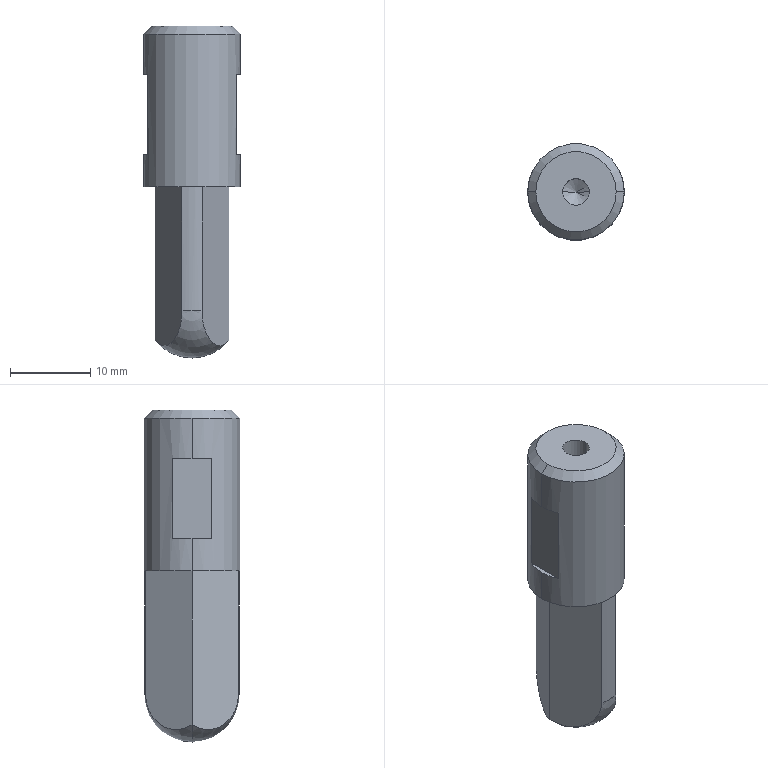Part | SolidWorks | features ICE 3, Chamfer 1, Extrusion 1, HoleWzd 1, Revolution 1 | 1 solid | 24 faces | box 12 x 12 x 41.3 mm | volume 3482 mm3 | plane 12 | cylinder 6 | cone 4 | sphere 2 | commonest cylinder face diameters 3.3 x2 11.8 x2 12 x2
STEP:
#1=CARTESIAN_POINT('',(5.,0.,35.4));
#2=VERTEX_POINT('',#1);
#3=CARTESIAN_POINT('',(-5.,0.,35.4));
#4=VERTEX_POINT('',#3);
#5=CARTESIAN_POINT('',(0.,0.,35.4));
#6=DIRECTION('',(0.,0.,1.));
#7=DIRECTION('',(1.,0.,0.));
#8=AXIS2_PLACEMENT_3D('',#5,#6,#7);
#9=CIRCLE('',#8,5.);
#10=EDGE_CURVE('',#2,#4,#9,.T.);
#11=ORIENTED_EDGE('',*,*,#10,.F.);
#12=CARTESIAN_POINT('',(6.,0.,34.4));
#13=VERTEX_POINT('',#12);
#14=CARTESIAN_POINT('',(5.,0.,35.4));
#15=DIRECTION('',(0.7071,0.,-0.7071));
#16=VECTOR('',#15,1000.);
#17=LINE('',#14,#16);
#18=EDGE_CURVE('',#2,#13,#17,.T.);
#19=ORIENTED_EDGE('',*,*,#18,.T.);
#20=CARTESIAN_POINT('',(-6.,0.,34.4));
#21=VERTEX_POINT('',#20);
#22=CARTESIAN_POINT('',(0.,0.,34.4));
#23=DIRECTION('',(0.,0.,-1.));
#24=DIRECTION('',(1.,0.,0.));
#25=AXIS2_PLACEMENT_3D('',#22,#23,#24);
#26=CIRCLE('',#25,6.);
#27=EDGE_CURVE('',#21,#13,#26,.T.);
#28=ORIENTED_EDGE('',*,*,#27,.F.);
#29=CARTESIAN_POINT('',(-5.,0.,35.4));
#30=DIRECTION('',(-0.7071,0.,-0.7071));
#31=VECTOR('',#30,1000.);
#32=LINE('',#29,#31);
#33=EDGE_CURVE('',#4,#21,#32,.T.);
#34=ORIENTED_EDGE('',*,*,#33,.F.);
#35=EDGE_LOOP('',(#11,#19,#28,#34));
#36=FACE_OUTER_BOUND('',#35,.T.);
#37=CARTESIAN_POINT('',(0.,0.,35.4));
#38=DIRECTION('',(0.,0.,-1.));
#39=DIRECTION('',(-1.,0.,0.));
#40=AXIS2_PLACEMENT_3D('',#37,#38,#39);
#41=CONICAL_SURFACE('',#40,5.,0.7854);
#42=ADVANCED_FACE('',(#36),#41,.T.);
#43=CARTESIAN_POINT('',(4.579,0.,-3.721));
#44=VERTEX_POINT('',#43);
#45=CARTESIAN_POINT('',(1.25,5.766,0.));
#46=VERTEX_POINT('',#45);
#47=CARTESIAN_POINT('',(3.434,1.983,0.));
#48=DIRECTION('',(0.866,0.5,0.));
#49=DIRECTION('',(0.5,-0.866,0.));
#50=AXIS2_PLACEMENT_3D('',#47,#48,#49);
#51=CIRCLE('',#50,4.369);
#52=EDGE_CURVE('',#44,#46,#51,.T.);
#53=ORIENTED_EDGE('',*,*,#52,.F.);
#54=CARTESIAN_POINT('',(0.,0.,-5.9));
#55=VERTEX_POINT('',#54);
#56=CARTESIAN_POINT('',(0.,0.,0.));
#57=DIRECTION('',(0.,1.,0.));
#58=DIRECTION('',(-1.,0.,0.));
#59=AXIS2_PLACEMENT_3D('',#56,#57,#58);
#60=CIRCLE('',#59,5.9);
#61=EDGE_CURVE('',#44,#55,#60,.T.);
#62=ORIENTED_EDGE('',*,*,#61,.T.);
#63=CARTESIAN_POINT('',(-4.579,0.,-3.721));
#64=VERTEX_POINT('',#63);
#65=CARTESIAN_POINT('',(0.,0.,0.));
#66=DIRECTION('',(0.,-1.,0.));
#67=DIRECTION('',(0.,0.,-1.));
#68=AXIS2_PLACEMENT_3D('',#65,#66,#67);
#69=CIRCLE('',#68,5.9);
#70=EDGE_CURVE('',#64,#55,#69,.T.);
#71=ORIENTED_EDGE('',*,*,#70,.F.);
#72=CARTESIAN_POINT('',(-1.25,5.766,0.));
#73=VERTEX_POINT('',#72);
#74=CARTESIAN_POINT('',(-3.434,1.983,0.));
#75=DIRECTION('',(-0.866,0.5,0.));
#76=DIRECTION('',(0.5,0.866,0.));
#77=AXIS2_PLACEMENT_3D('',#74,#75,#76);
#78=CIRCLE('',#77,4.369);
#79=EDGE_CURVE('',#73,#64,#78,.T.);
#80=ORIENTED_EDGE('',*,*,#79,.F.);
#81=CARTESIAN_POINT('',(0.,0.,0.));
#82=DIRECTION('',(0.,0.,-1.));
#83=DIRECTION('',(-1.,0.,0.));
#84=AXIS2_PLACEMENT_3D('',#81,#82,#83);
#85=CIRCLE('',#84,5.9);
#86=EDGE_CURVE('',#73,#46,#85,.T.);
#87=ORIENTED_EDGE('',*,*,#86,.T.);
#88=EDGE_LOOP('',(#53,#62,#71,#80,#87));
#89=FACE_OUTER_BOUND('',#88,.T.);
#90=CARTESIAN_POINT('',(0.,0.,0.));
#91=DIRECTION('',(0.,1.,0.));
#92=DIRECTION('',(-1.,0.,0.));
#93=AXIS2_PLACEMENT_3D('',#90,#91,#92);
#94=SPHERICAL_SURFACE('',#93,5.9);
#95=ADVANCED_FACE('',(#89),#94,.T.);
#96=CARTESIAN_POINT('',(6.,0.,15.4));
#97=VERTEX_POINT('',#96);
#98=CARTESIAN_POINT('',(-6.,0.,15.4));
#99=VERTEX_POINT('',#98);
#100=CARTESIAN_POINT('',(0.,0.,15.4));
#101=DIRECTION('',(0.,0.,1.));
#102=DIRECTION('',(1.,0.,0.));
#103=AXIS2_PLACEMENT_3D('',#100,#101,#102);
#104=CIRCLE('',#103,6.);
#105=EDGE_CURVE('',#97,#99,#104,.T.);
#106=ORIENTED_EDGE('',*,*,#105,.T.);
#107=CARTESIAN_POINT('',(-6.,0.,19.4));
#108=VERTEX_POINT('',#107);
#109=CARTESIAN_POINT('',(-6.,0.,15.4));
#110=DIRECTION('',(0.,0.,1.));
#111=VECTOR('',#110,1000.);
#112=LINE('',#109,#111);
#113=EDGE_CURVE('',#99,#108,#112,.T.);
#114=ORIENTED_EDGE('',*,*,#113,.T.);
#115=CARTESIAN_POINT('',(-5.5,2.398,19.4));
#116=VERTEX_POINT('',#115);
#117=CARTESIAN_POINT('',(0.,0.,19.4));
#118=DIRECTION('',(0.,0.,1.));
#119=DIRECTION('',(-1.,0.,0.));
#120=AXIS2_PLACEMENT_3D('',#117,#118,#119);
#121=CIRCLE('',#120,6.);
#122=EDGE_CURVE('',#116,#108,#121,.T.);
#123=ORIENTED_EDGE('',*,*,#122,.F.);
#124=CARTESIAN_POINT('',(-5.5,2.398,29.4));
#125=VERTEX_POINT('',#124);
#126=CARTESIAN_POINT('',(-5.5,2.398,15.4));
#127=DIRECTION('',(0.,0.,-1.));
#128=VECTOR('',#127,1000.);
#129=LINE('',#126,#128);
#130=EDGE_CURVE('',#125,#116,#129,.T.);
#131=ORIENTED_EDGE('',*,*,#130,.F.);
#132=CARTESIAN_POINT('',(-6.,0.,29.4));
#133=VERTEX_POINT('',#132);
#134=CARTESIAN_POINT('',(0.,0.,29.4));
#135=DIRECTION('',(0.,0.,-1.));
#136=DIRECTION('',(1.,0.,0.));
#137=AXIS2_PLACEMENT_3D('',#134,#135,#136);
#138=CIRCLE('',#137,6.);
#139=EDGE_CURVE('',#133,#125,#138,.T.);
#140=ORIENTED_EDGE('',*,*,#139,.F.);
#141=CARTESIAN_POINT('',(-6.,0.,15.4));
#142=DIRECTION('',(0.,0.,1.));
#143=VECTOR('',#142,1000.);
#144=LINE('',#141,#143);
#145=EDGE_CURVE('',#133,#21,#144,.T.);
#146=ORIENTED_EDGE('',*,*,#145,.T.);
#147=ORIENTED_EDGE('',*,*,#27,.T.);
#148=CARTESIAN_POINT('',(6.,0.,29.4));
#149=VERTEX_POINT('',#148);
#150=CARTESIAN_POINT('',(6.,0.,15.4));
#151=DIRECTION('',(0.,0.,1.));
#152=VECTOR('',#151,1000.);
#153=LINE('',#150,#152);
#154=EDGE_CURVE('',#149,#13,#153,.T.);
#155=ORIENTED_EDGE('',*,*,#154,.F.);
#156=CARTESIAN_POINT('',(5.5,2.398,29.4));
#157=VERTEX_POINT('',#156);
#158=CARTESIAN_POINT('',(0.,0.,29.4));
#159=DIRECTION('',(0.,0.,-1.));
#160=DIRECTION('',(1.,0.,0.));
#161=AXIS2_PLACEMENT_3D('',#158,#159,#160);
#162=CIRCLE('',#161,6.);
#163=EDGE_CURVE('',#157,#149,#162,.T.);
#164=ORIENTED_EDGE('',*,*,#163,.F.);
#165=CARTESIAN_POINT('',(5.5,2.398,19.4));
#166=VERTEX_POINT('',#165);
#167=CARTESIAN_POINT('',(5.5,2.398,15.4));
#168=DIRECTION('',(0.,0.,1.));
#169=VECTOR('',#168,1000.);
#170=LINE('',#167,#169);
#171=EDGE_CURVE('',#166,#157,#170,.T.);
#172=ORIENTED_EDGE('',*,*,#171,.F.);
#173=CARTESIAN_POINT('',(6.,0.,19.4));
#174=VERTEX_POINT('',#173);
#175=CARTESIAN_POINT('',(0.,0.,19.4));
#176=DIRECTION('',(0.,0.,1.));
#177=DIRECTION('',(-1.,0.,0.));
#178=AXIS2_PLACEMENT_3D('',#175,#176,#177);
#179=CIRCLE('',#178,6.);
#180=EDGE_CURVE('',#174,#166,#179,.T.);
#181=ORIENTED_EDGE('',*,*,#180,.F.);
#182=CARTESIAN_POINT('',(6.,0.,15.4));
#183=DIRECTION('',(0.,0.,1.));
#184=VECTOR('',#183,1000.);
#185=LINE('',#182,#184);
#186=EDGE_CURVE('',#97,#174,#185,.T.);
#187=ORIENTED_EDGE('',*,*,#186,.F.);
#188=EDGE_LOOP('',(#106,#114,#123,#131,#140,#146,#147,#155,#164,#172,#181,#187));
#189=FACE_OUTER_BOUND('',#188,.T.);
#190=CARTESIAN_POINT('',(0.,0.,15.4));
#191=DIRECTION('',(0.,0.,1.));
#192=DIRECTION('',(1.,0.,0.));
#193=AXIS2_PLACEMENT_3D('',#190,#191,#192);
#194=CYLINDRICAL_SURFACE('',#193,6.);
#195=ADVANCED_FACE('',(#189),#194,.T.);
#196=CARTESIAN_POINT('',(-1.65,0.,25.3));
#197=VERTEX_POINT('',#196);
#198=CARTESIAN_POINT('',(1.65,0.,25.3));
#199=VERTEX_POINT('',#198);
#200=CARTESIAN_POINT('',(0.,0.,25.3));
#201=DIRECTION('',(0.,0.,1.));
#202=DIRECTION('',(1.,0.,0.));
#203=AXIS2_PLACEMENT_3D('',#200,#201,#202);
#204=CIRCLE('',#203,1.65);
#205=EDGE_CURVE('',#197,#199,#204,.T.);
#206=ORIENTED_EDGE('',*,*,#205,.F.);
#207=CARTESIAN_POINT('',(-1.65,0.,35.4));
#208=VERTEX_POINT('',#207);
#209=CARTESIAN_POINT('',(-1.65,0.,35.4));
#210=DIRECTION('',(0.,0.,1.));
#211=VECTOR('',#210,1000.);
#212=LINE('',#209,#211);
#213=EDGE_CURVE('',#197,#208,#212,.T.);
#214=ORIENTED_EDGE('',*,*,#213,.T.);
#215=CARTESIAN_POINT('',(1.65,0.,35.4));
#216=VERTEX_POINT('',#215);
#217=CARTESIAN_POINT('',(0.,0.,35.4));
#218=DIRECTION('',(0.,0.,1.));
#219=DIRECTION('',(1.,0.,0.));
#220=AXIS2_PLACEMENT_3D('',#217,#218,#219);
#221=CIRCLE('',#220,1.65);
#222=EDGE_CURVE('',#208,#216,#221,.T.);
#223=ORIENTED_EDGE('',*,*,#222,.T.);
#224=CARTESIAN_POINT('',(1.65,0.,35.4));
#225=DIRECTION('',(0.,0.,1.));
#226=VECTOR('',#225,1000.);
#227=LINE('',#224,#226);
#228=EDGE_CURVE('',#199,#216,#227,.T.);
#229=ORIENTED_EDGE('',*,*,#228,.F.);
#230=EDGE_LOOP('',(#206,#214,#223,#229));
#231=FACE_OUTER_BOUND('',#230,.T.);
#232=CARTESIAN_POINT('',(0.,0.,35.4));
#233=DIRECTION('',(0.,0.,1.));
#234=DIRECTION('',(1.,0.,0.));
#235=AXIS2_PLACEMENT_3D('',#232,#233,#234);
#236=CYLINDRICAL_SURFACE('',#235,1.65);
#237=ADVANCED_FACE('',(#231),#236,.F.);
#238=CARTESIAN_POINT('',(0.,0.,24.309));
#239=VERTEX_POINT('',#238);
#240=CARTESIAN_POINT('',(1.65,0.,25.3));
#241=DIRECTION('',(0.8572,0.,0.515));
#242=VECTOR('',#241,1000.);
#243=LINE('',#240,#242);
#244=EDGE_CURVE('',#239,#199,#243,.T.);
#245=ORIENTED_EDGE('',*,*,#244,.F.);
#246=CARTESIAN_POINT('',(-1.65,0.,25.3));
#247=DIRECTION('',(-0.8572,0.,0.515));
#248=VECTOR('',#247,1000.);
#249=LINE('',#246,#248);
#250=EDGE_CURVE('',#239,#197,#249,.T.);
#251=ORIENTED_EDGE('',*,*,#250,.T.);
#252=ORIENTED_EDGE('',*,*,#205,.T.);
#253=EDGE_LOOP('',(#245,#251,#252));
#254=FACE_OUTER_BOUND('',#253,.T.);
#255=CARTESIAN_POINT('',(0.,0.,25.3));
#256=DIRECTION('',(0.,0.,1.));
#257=DIRECTION('',(1.,0.,0.));
#258=AXIS2_PLACEMENT_3D('',#255,#256,#257);
#259=CONICAL_SURFACE('',#258,1.65,1.03);
#260=ADVANCED_FACE('',(#254),#259,.F.);
#261=CARTESIAN_POINT('',(1.25,5.766,15.4));
#262=VERTEX_POINT('',#261);
#263=CARTESIAN_POINT('',(-1.25,5.766,15.4));
#264=VERTEX_POINT('',#263);
#265=CARTESIAN_POINT('',(0.,0.,15.4));
#266=DIRECTION('',(0.,0.,1.));
#267=DIRECTION('',(1.,0.,0.));
#268=AXIS2_PLACEMENT_3D('',#265,#266,#267);
#269=CIRCLE('',#268,5.9);
#270=EDGE_CURVE('',#262,#264,#269,.T.);
#271=ORIENTED_EDGE('',*,*,#270,.F.);
#272=CARTESIAN_POINT('',(1.25,5.766,35.4));
#273=DIRECTION('',(0.,0.,-1.));
#274=VECTOR('',#273,1000.);
#275=LINE('',#272,#274);
#276=EDGE_CURVE('',#262,#46,#275,.T.);
#277=ORIENTED_EDGE('',*,*,#276,.T.);
#278=ORIENTED_EDGE('',*,*,#86,.F.);
#279=CARTESIAN_POINT('',(-1.25,5.766,35.4));
#280=DIRECTION('',(0.,0.,1.));
#281=VECTOR('',#280,1000.);
#282=LINE('',#279,#281);
#283=EDGE_CURVE('',#73,#264,#282,.T.);
#284=ORIENTED_EDGE('',*,*,#283,.T.);
#285=EDGE_LOOP('',(#271,#277,#278,#284));
#286=FACE_OUTER_BOUND('',#285,.T.);
#287=CARTESIAN_POINT('',(0.,0.,35.4));
#288=DIRECTION('',(0.,0.,-1.));
#289=DIRECTION('',(-1.,0.,0.));
#290=AXIS2_PLACEMENT_3D('',#287,#288,#289);
#291=CYLINDRICAL_SURFACE('',#290,5.9);
#292=ADVANCED_FACE('',(#286),#291,.T.);
#293=CARTESIAN_POINT('',(0.,0.,35.4));
#294=DIRECTION('',(0.,0.,1.));
#295=DIRECTION('',(1.,0.,0.));
#296=AXIS2_PLACEMENT_3D('',#293,#294,#295);
#297=CIRCLE('',#296,5.);
#298=EDGE_CURVE('',#4,#2,#297,.T.);
#299=ORIENTED_EDGE('',*,*,#298,.T.);
#300=ORIENTED_EDGE('',*,*,#10,.T.);
#301=EDGE_LOOP('',(#299,#300));
#302=FACE_OUTER_BOUND('',#301,.T.);
#303=CARTESIAN_POINT('',(0.,0.,35.4));
#304=DIRECTION('',(0.,0.,1.));
#305=DIRECTION('',(1.,0.,0.));
#306=AXIS2_PLACEMENT_3D('',#303,#304,#305);
#307=CIRCLE('',#306,1.65);
#308=EDGE_CURVE('',#216,#208,#307,.T.);
#309=ORIENTED_EDGE('',*,*,#308,.F.);
#310=ORIENTED_EDGE('',*,*,#222,.F.);
#311=EDGE_LOOP('',(#309,#310));
#312=FACE_BOUND('',#311,.T.);
#313=CARTESIAN_POINT('',(0.,0.,35.4));
#314=DIRECTION('',(0.,0.,1.));
#315=DIRECTION('',(1.,0.,0.));
#316=AXIS2_PLACEMENT_3D('',#313,#314,#315);
#317=PLANE('',#316);
#318=ADVANCED_FACE('',(#302,#312),#317,.T.);
#319=ORIENTED_EDGE('',*,*,#250,.F.);
#320=ORIENTED_EDGE('',*,*,#244,.T.);
#321=CARTESIAN_POINT('',(0.,0.,25.3));
#322=DIRECTION('',(0.,0.,1.));
#323=DIRECTION('',(1.,0.,0.));
#324=AXIS2_PLACEMENT_3D('',#321,#322,#323);
#325=CIRCLE('',#324,1.65);
#326=EDGE_CURVE('',#199,#197,#325,.T.);
#327=ORIENTED_EDGE('',*,*,#326,.T.);
#328=EDGE_LOOP('',(#319,#320,#327));
#329=FACE_OUTER_BOUND('',#328,.T.);
#330=CARTESIAN_POINT('',(0.,0.,25.3));
#331=DIRECTION('',(0.,0.,1.));
#332=DIRECTION('',(1.,0.,0.));
#333=AXIS2_PLACEMENT_3D('',#330,#331,#332);
#334=CONICAL_SURFACE('',#333,1.65,1.03);
#335=ADVANCED_FACE('',(#329),#334,.F.);
#336=ORIENTED_EDGE('',*,*,#213,.F.);
#337=ORIENTED_EDGE('',*,*,#326,.F.);
#338=ORIENTED_EDGE('',*,*,#228,.T.);
#339=ORIENTED_EDGE('',*,*,#308,.T.);
#340=EDGE_LOOP('',(#336,#337,#338,#339));
#341=FACE_OUTER_BOUND('',#340,.T.);
#342=CARTESIAN_POINT('',(0.,0.,35.4));
#343=DIRECTION('',(0.,0.,1.));
#344=DIRECTION('',(1.,0.,0.));
#345=AXIS2_PLACEMENT_3D('',#342,#343,#344);
#346=CYLINDRICAL_SURFACE('',#345,1.65);
#347=ADVANCED_FACE('',(#341),#346,.F.);
#348=ORIENTED_EDGE('',*,*,#113,.F.);
#349=CARTESIAN_POINT('',(0.,0.,15.4));
#350=DIRECTION('',(0.,0.,1.));
#351=DIRECTION('',(1.,0.,0.));
#352=AXIS2_PLACEMENT_3D('',#349,#350,#351);
#353=CIRCLE('',#352,6.);
#354=EDGE_CURVE('',#99,#97,#353,.T.);
#355=ORIENTED_EDGE('',*,*,#354,.T.);
#356=ORIENTED_EDGE('',*,*,#186,.T.);
#357=CARTESIAN_POINT('',(5.5,-2.398,19.4));
#358=VERTEX_POINT('',#357);
#359=CARTESIAN_POINT('',(0.,0.,19.4));
#360=DIRECTION('',(0.,0.,1.));
#361=DIRECTION('',(-1.,0.,0.));
#362=AXIS2_PLACEMENT_3D('',#359,#360,#361);
#363=CIRCLE('',#362,6.);
#364=EDGE_CURVE('',#358,#174,#363,.T.);
#365=ORIENTED_EDGE('',*,*,#364,.F.);
#366=CARTESIAN_POINT('',(5.5,-2.398,29.4));
#367=VERTEX_POINT('',#366);
#368=CARTESIAN_POINT('',(5.5,-2.398,15.4));
#369=DIRECTION('',(0.,0.,-1.));
#370=VECTOR('',#369,1000.);
#371=LINE('',#368,#370);
#372=EDGE_CURVE('',#367,#358,#371,.T.);
#373=ORIENTED_EDGE('',*,*,#372,.F.);
#374=CARTESIAN_POINT('',(0.,0.,29.4));
#375=DIRECTION('',(0.,0.,-1.));
#376=DIRECTION('',(1.,0.,0.));
#377=AXIS2_PLACEMENT_3D('',#374,#375,#376);
#378=CIRCLE('',#377,6.);
#379=EDGE_CURVE('',#149,#367,#378,.T.);
#380=ORIENTED_EDGE('',*,*,#379,.F.);
#381=ORIENTED_EDGE('',*,*,#154,.T.);
#382=CARTESIAN_POINT('',(0.,0.,34.4));
#383=DIRECTION('',(0.,0.,-1.));
#384=DIRECTION('',(1.,0.,0.));
#385=AXIS2_PLACEMENT_3D('',#382,#383,#384);
#386=CIRCLE('',#385,6.);
#387=EDGE_CURVE('',#13,#21,#386,.T.);
#388=ORIENTED_EDGE('',*,*,#387,.T.);
#389=ORIENTED_EDGE('',*,*,#145,.F.);
#390=CARTESIAN_POINT('',(-5.5,-2.398,29.4));
#391=VERTEX_POINT('',#390);
#392=CARTESIAN_POINT('',(0.,0.,29.4));
#393=DIRECTION('',(0.,0.,-1.));
#394=DIRECTION('',(1.,0.,0.));
#395=AXIS2_PLACEMENT_3D('',#392,#393,#394);
#396=CIRCLE('',#395,6.);
#397=EDGE_CURVE('',#391,#133,#396,.T.);
#398=ORIENTED_EDGE('',*,*,#397,.F.);
#399=CARTESIAN_POINT('',(-5.5,-2.398,19.4));
#400=VERTEX_POINT('',#399);
#401=CARTESIAN_POINT('',(-5.5,-2.398,15.4));
#402=DIRECTION('',(0.,0.,1.));
#403=VECTOR('',#402,1000.);
#404=LINE('',#401,#403);
#405=EDGE_CURVE('',#400,#391,#404,.T.);
#406=ORIENTED_EDGE('',*,*,#405,.F.);
#407=CARTESIAN_POINT('',(0.,0.,19.4));
#408=DIRECTION('',(0.,0.,1.));
#409=DIRECTION('',(-1.,0.,0.));
#410=AXIS2_PLACEMENT_3D('',#407,#408,#409);
#411=CIRCLE('',#410,6.);
#412=EDGE_CURVE('',#108,#400,#411,.T.);
#413=ORIENTED_EDGE('',*,*,#412,.F.);
#414=EDGE_LOOP('',(#348,#355,#356,#365,#373,#380,#381,#388,#389,#398,#406,#413));
#415=FACE_OUTER_BOUND('',#414,.T.);
#416=CARTESIAN_POINT('',(0.,0.,15.4));
#417=DIRECTION('',(0.,0.,1.));
#418=DIRECTION('',(1.,0.,0.));
#419=AXIS2_PLACEMENT_3D('',#416,#417,#418);
#420=CYLINDRICAL_SURFACE('',#419,6.);
#421=ADVANCED_FACE('',(#415),#420,.T.);
#422=ORIENTED_EDGE('',*,*,#270,.T.);
#423=CARTESIAN_POINT('',(-4.579,0.,15.4));
#424=VERTEX_POINT('',#423);
#425=CARTESIAN_POINT('',(-1.25,5.766,15.4));
#426=DIRECTION('',(0.5,0.866,0.));
#427=VECTOR('',#426,1000.);
#428=LINE('',#425,#427);
#429=EDGE_CURVE('',#424,#264,#428,.T.);
#430=ORIENTED_EDGE('',*,*,#429,.F.);
#431=CARTESIAN_POINT('',(-1.25,-5.766,15.4));
#432=VERTEX_POINT('',#431);
#433=CARTESIAN_POINT('',(-4.579,0.,15.4));
#434=DIRECTION('',(-0.5,0.866,0.));
#435=VECTOR('',#434,1000.);
#436=LINE('',#433,#435);
#437=EDGE_CURVE('',#432,#424,#436,.T.);
#438=ORIENTED_EDGE('',*,*,#437,.F.);
#439=CARTESIAN_POINT('',(1.25,-5.766,15.4));
#440=VERTEX_POINT('',#439);
#441=CARTESIAN_POINT('',(0.,0.,15.4));
#442=DIRECTION('',(0.,0.,1.));
#443=DIRECTION('',(1.,0.,0.));
#444=AXIS2_PLACEMENT_3D('',#441,#442,#443);
#445=CIRCLE('',#444,5.9);
#446=EDGE_CURVE('',#432,#440,#445,.T.);
#447=ORIENTED_EDGE('',*,*,#446,.T.);
#448=CARTESIAN_POINT('',(4.579,0.,15.4));
#449=VERTEX_POINT('',#448);
#450=CARTESIAN_POINT('',(4.579,0.,15.4));
#451=DIRECTION('',(-0.5,-0.866,0.));
#452=VECTOR('',#451,1000.);
#453=LINE('',#450,#452);
#454=EDGE_CURVE('',#449,#440,#453,.T.);
#455=ORIENTED_EDGE('',*,*,#454,.F.);
#456=CARTESIAN_POINT('',(1.25,5.766,15.4));
#457=DIRECTION('',(0.5,-0.866,0.));
#458=VECTOR('',#457,1000.);
#459=LINE('',#456,#458);
#460=EDGE_CURVE('',#262,#449,#459,.T.);
#461=ORIENTED_EDGE('',*,*,#460,.F.);
#462=EDGE_LOOP('',(#422,#430,#438,#447,#455,#461));
#463=FACE_BOUND('',#462,.T.);
#464=ORIENTED_EDGE('',*,*,#105,.F.);
#465=ORIENTED_EDGE('',*,*,#354,.F.);
#466=EDGE_LOOP('',(#464,#465));
#467=FACE_OUTER_BOUND('',#466,.T.);
#468=CARTESIAN_POINT('',(0.,0.,15.4));
#469=DIRECTION('',(0.,0.,1.));
#470=DIRECTION('',(1.,0.,0.));
#471=AXIS2_PLACEMENT_3D('',#468,#469,#470);
#472=PLANE('',#471);
#473=ADVANCED_FACE('',(#463,#467),#472,.F.);
#474=ORIENTED_EDGE('',*,*,#61,.F.);
#475=CARTESIAN_POINT('',(1.25,-5.766,0.));
#476=VERTEX_POINT('',#475);
#477=CARTESIAN_POINT('',(3.434,-1.983,0.));
#478=DIRECTION('',(0.866,-0.5,0.));
#479=DIRECTION('',(-0.5,-0.866,0.));
#480=AXIS2_PLACEMENT_3D('',#477,#478,#479);
#481=CIRCLE('',#480,4.369);
#482=EDGE_CURVE('',#476,#44,#481,.T.);
#483=ORIENTED_EDGE('',*,*,#482,.F.);
#484=CARTESIAN_POINT('',(-1.25,-5.766,0.));
#485=VERTEX_POINT('',#484);
#486=CARTESIAN_POINT('',(0.,0.,0.));
#487=DIRECTION('',(0.,0.,-1.));
#488=DIRECTION('',(-1.,0.,0.));
#489=AXIS2_PLACEMENT_3D('',#486,#487,#488);
#490=CIRCLE('',#489,5.9);
#491=EDGE_CURVE('',#476,#485,#490,.T.);
#492=ORIENTED_EDGE('',*,*,#491,.T.);
#493=CARTESIAN_POINT('',(-3.434,-1.983,0.));
#494=DIRECTION('',(-0.866,-0.5,0.));
#495=DIRECTION('',(-0.5,0.866,0.));
#496=AXIS2_PLACEMENT_3D('',#493,#494,#495);
#497=CIRCLE('',#496,4.369);
#498=EDGE_CURVE('',#64,#485,#497,.T.);
#499=ORIENTED_EDGE('',*,*,#498,.F.);
#500=ORIENTED_EDGE('',*,*,#70,.T.);
#501=EDGE_LOOP('',(#474,#483,#492,#499,#500));
#502=FACE_OUTER_BOUND('',#501,.T.);
#503=CARTESIAN_POINT('',(0.,0.,0.));
#504=DIRECTION('',(0.,1.,0.));
#505=DIRECTION('',(-1.,0.,0.));
#506=AXIS2_PLACEMENT_3D('',#503,#504,#505);
#507=SPHERICAL_SURFACE('',#506,5.9);
#508=ADVANCED_FACE('',(#502),#507,.T.);
#509=ORIENTED_EDGE('',*,*,#491,.F.);
#510=CARTESIAN_POINT('',(1.25,-5.766,35.4));
#511=DIRECTION('',(0.,0.,1.));
#512=VECTOR('',#511,1000.);
#513=LINE('',#510,#512);
#514=EDGE_CURVE('',#476,#440,#513,.T.);
#515=ORIENTED_EDGE('',*,*,#514,.T.);
#516=ORIENTED_EDGE('',*,*,#446,.F.);
#517=CARTESIAN_POINT('',(-1.25,-5.766,35.4));
#518=DIRECTION('',(0.,0.,-1.));
#519=VECTOR('',#518,1000.);
#520=LINE('',#517,#519);
#521=EDGE_CURVE('',#432,#485,#520,.T.);
#522=ORIENTED_EDGE('',*,*,#521,.T.);
#523=EDGE_LOOP('',(#509,#515,#516,#522));
#524=FACE_OUTER_BOUND('',#523,.T.);
#525=CARTESIAN_POINT('',(0.,0.,35.4));
#526=DIRECTION('',(0.,0.,-1.));
#527=DIRECTION('',(-1.,0.,0.));
#528=AXIS2_PLACEMENT_3D('',#525,#526,#527);
#529=CYLINDRICAL_SURFACE('',#528,5.9);
#530=ADVANCED_FACE('',(#524),#529,.T.);
#531=ORIENTED_EDGE('',*,*,#18,.F.);
#532=ORIENTED_EDGE('',*,*,#298,.F.);
#533=ORIENTED_EDGE('',*,*,#33,.T.);
#534=ORIENTED_EDGE('',*,*,#387,.F.);
#535=EDGE_LOOP('',(#531,#532,#533,#534));
#536=FACE_OUTER_BOUND('',#535,.T.);
#537=CARTESIAN_POINT('',(0.,0.,35.4));
#538=DIRECTION('',(0.,0.,-1.));
#539=DIRECTION('',(-1.,0.,0.));
#540=AXIS2_PLACEMENT_3D('',#537,#538,#539);
#541=CONICAL_SURFACE('',#540,5.,0.7854);
#542=ADVANCED_FACE('',(#536),#541,.T.);
#543=ORIENTED_EDGE('',*,*,#163,.T.);
#544=ORIENTED_EDGE('',*,*,#379,.T.);
#545=CARTESIAN_POINT('',(5.5,-6.,29.4));
#546=DIRECTION('',(0.,1.,0.));
#547=VECTOR('',#546,1000.);
#548=LINE('',#545,#547);
#549=EDGE_CURVE('',#367,#157,#548,.T.);
#550=ORIENTED_EDGE('',*,*,#549,.T.);
#551=EDGE_LOOP('',(#543,#544,#550));
#552=FACE_OUTER_BOUND('',#551,.T.);
#553=CARTESIAN_POINT('',(7.526,-6.,29.4));
#554=DIRECTION('',(0.,0.,1.));
#555=DIRECTION('',(1.,0.,0.));
#556=AXIS2_PLACEMENT_3D('',#553,#554,#555);
#557=PLANE('',#556);
#558=ADVANCED_FACE('',(#552),#557,.F.);
#559=ORIENTED_EDGE('',*,*,#372,.T.);
#560=CARTESIAN_POINT('',(5.5,-6.,19.4));
#561=DIRECTION('',(0.,1.,0.));
#562=VECTOR('',#561,1000.);
#563=LINE('',#560,#562);
#564=EDGE_CURVE('',#358,#166,#563,.T.);
#565=ORIENTED_EDGE('',*,*,#564,.T.);
#566=ORIENTED_EDGE('',*,*,#171,.T.);
#567=ORIENTED_EDGE('',*,*,#549,.F.);
#568=EDGE_LOOP('',(#559,#565,#566,#567));
#569=FACE_OUTER_BOUND('',#568,.T.);
#570=CARTESIAN_POINT('',(5.5,-6.,19.4));
#571=DIRECTION('',(-1.,0.,0.));
#572=DIRECTION('',(0.,0.,1.));
#573=AXIS2_PLACEMENT_3D('',#570,#571,#572);
#574=PLANE('',#573);
#575=ADVANCED_FACE('',(#569),#574,.F.);
#576=ORIENTED_EDGE('',*,*,#364,.T.);
#577=ORIENTED_EDGE('',*,*,#180,.T.);
#578=ORIENTED_EDGE('',*,*,#564,.F.);
#579=EDGE_LOOP('',(#576,#577,#578));
#580=FACE_OUTER_BOUND('',#579,.T.);
#581=CARTESIAN_POINT('',(7.526,-6.,19.4));
#582=DIRECTION('',(0.,0.,-1.));
#583=DIRECTION('',(-1.,0.,0.));
#584=AXIS2_PLACEMENT_3D('',#581,#582,#583);
#585=PLANE('',#584);
#586=ADVANCED_FACE('',(#580),#585,.F.);
#587=ORIENTED_EDGE('',*,*,#122,.T.);
#588=ORIENTED_EDGE('',*,*,#412,.T.);
#589=CARTESIAN_POINT('',(-5.5,-6.,19.4));
#590=DIRECTION('',(0.,1.,0.));
#591=VECTOR('',#590,1000.);
#592=LINE('',#589,#591);
#593=EDGE_CURVE('',#400,#116,#592,.T.);
#594=ORIENTED_EDGE('',*,*,#593,.T.);
#595=EDGE_LOOP('',(#587,#588,#594));
#596=FACE_OUTER_BOUND('',#595,.T.);
#597=CARTESIAN_POINT('',(-7.526,-6.,19.4));
#598=DIRECTION('',(0.,0.,-1.));
#599=DIRECTION('',(-1.,0.,0.));
#600=AXIS2_PLACEMENT_3D('',#597,#598,#599);
#601=PLANE('',#600);
#602=ADVANCED_FACE('',(#596),#601,.F.);
#603=ORIENTED_EDGE('',*,*,#130,.T.);
#604=ORIENTED_EDGE('',*,*,#593,.F.);
#605=ORIENTED_EDGE('',*,*,#405,.T.);
#606=CARTESIAN_POINT('',(-5.5,-6.,29.4));
#607=DIRECTION('',(0.,1.,0.));
#608=VECTOR('',#607,1000.);
#609=LINE('',#606,#608);
#610=EDGE_CURVE('',#391,#125,#609,.T.);
#611=ORIENTED_EDGE('',*,*,#610,.T.);
#612=EDGE_LOOP('',(#603,#604,#605,#611));
#613=FACE_OUTER_BOUND('',#612,.T.);
#614=CARTESIAN_POINT('',(-5.5,-6.,19.4));
#615=DIRECTION('',(1.,0.,0.));
#616=DIRECTION('',(0.,0.,-1.));
#617=AXIS2_PLACEMENT_3D('',#614,#615,#616);
#618=PLANE('',#617);
#619=ADVANCED_FACE('',(#613),#618,.F.);
#620=ORIENTED_EDGE('',*,*,#397,.T.);
#621=ORIENTED_EDGE('',*,*,#139,.T.);
#622=ORIENTED_EDGE('',*,*,#610,.F.);
#623=EDGE_LOOP('',(#620,#621,#622));
#624=FACE_OUTER_BOUND('',#623,.T.);
#625=CARTESIAN_POINT('',(-7.526,-6.,29.4));
#626=DIRECTION('',(0.,0.,1.));
#627=DIRECTION('',(1.,0.,0.));
#628=AXIS2_PLACEMENT_3D('',#625,#626,#627);
#629=PLANE('',#628);
#630=ADVANCED_FACE('',(#624),#629,.F.);
#631=ORIENTED_EDGE('',*,*,#79,.T.);
#632=CARTESIAN_POINT('',(-4.579,0.,-5.9));
#633=DIRECTION('',(0.,0.,1.));
#634=VECTOR('',#633,1000.);
#635=LINE('',#632,#634);
#636=EDGE_CURVE('',#64,#424,#635,.T.);
#637=ORIENTED_EDGE('',*,*,#636,.T.);
#638=ORIENTED_EDGE('',*,*,#429,.T.);
#639=ORIENTED_EDGE('',*,*,#283,.F.);
#640=EDGE_LOOP('',(#631,#637,#638,#639));
#641=FACE_OUTER_BOUND('',#640,.T.);
#642=CARTESIAN_POINT('',(-1.25,5.766,-5.9));
#643=DIRECTION('',(0.866,-0.5,0.));
#644=DIRECTION('',(0.5,0.866,0.));
#645=AXIS2_PLACEMENT_3D('',#642,#643,#644);
#646=PLANE('',#645);
#647=ADVANCED_FACE('',(#641),#646,.F.);
#648=ORIENTED_EDGE('',*,*,#498,.T.);
#649=ORIENTED_EDGE('',*,*,#521,.F.);
#650=ORIENTED_EDGE('',*,*,#437,.T.);
#651=ORIENTED_EDGE('',*,*,#636,.F.);
#652=EDGE_LOOP('',(#648,#649,#650,#651));
#653=FACE_OUTER_BOUND('',#652,.T.);
#654=CARTESIAN_POINT('',(-4.579,0.,-5.9));
#655=DIRECTION('',(0.866,0.5,0.));
#656=DIRECTION('',(-0.5,0.866,0.));
#657=AXIS2_PLACEMENT_3D('',#654,#655,#656);
#658=PLANE('',#657);
#659=ADVANCED_FACE('',(#653),#658,.F.);
#660=ORIENTED_EDGE('',*,*,#52,.T.);
#661=ORIENTED_EDGE('',*,*,#276,.F.);
#662=ORIENTED_EDGE('',*,*,#460,.T.);
#663=CARTESIAN_POINT('',(4.579,0.,-5.9));
#664=DIRECTION('',(0.,0.,1.));
#665=VECTOR('',#664,1000.);
#666=LINE('',#663,#665);
#667=EDGE_CURVE('',#44,#449,#666,.T.);
#668=ORIENTED_EDGE('',*,*,#667,.F.);
#669=EDGE_LOOP('',(#660,#661,#662,#668));
#670=FACE_OUTER_BOUND('',#669,.T.);
#671=CARTESIAN_POINT('',(1.25,5.766,-5.9));
#672=DIRECTION('',(-0.866,-0.5,0.));
#673=DIRECTION('',(0.5,-0.866,0.));
#674=AXIS2_PLACEMENT_3D('',#671,#672,#673);
#675=PLANE('',#674);
#676=ADVANCED_FACE('',(#670),#675,.F.);
#677=ORIENTED_EDGE('',*,*,#482,.T.);
#678=ORIENTED_EDGE('',*,*,#667,.T.);
#679=ORIENTED_EDGE('',*,*,#454,.T.);
#680=ORIENTED_EDGE('',*,*,#514,.F.);
#681=EDGE_LOOP('',(#677,#678,#679,#680));
#682=FACE_OUTER_BOUND('',#681,.T.);
#683=CARTESIAN_POINT('',(4.579,0.,-5.9));
#684=DIRECTION('',(-0.866,0.5,0.));
#685=DIRECTION('',(-0.5,-0.866,0.));
#686=AXIS2_PLACEMENT_3D('',#683,#684,#685);
#687=PLANE('',#686);
#688=ADVANCED_FACE('',(#682),#687,.F.);
#689=CLOSED_SHELL('',(#42,#95,#195,#237,#260,#292,#318,#335,#347,#421,#473,#508,#530,#542,#558,#575,#586,#602,#619,#630,#647,#659,#676,#688));
#690=MANIFOLD_SOLID_BREP('',#689);
#691=CARTESIAN_POINT('',(0.,0.,0.));
#692=DIRECTION('',(0.,0.,1.));
#693=DIRECTION('',(1.,0.,0.));
#694=AXIS2_PLACEMENT_3D('',#691,#692,#693);
#695=(LENGTH_UNIT()NAMED_UNIT(*)SI_UNIT(.MILLI.,.METRE.));
#696=UNCERTAINTY_MEASURE_WITH_UNIT(LENGTH_MEASURE(0.00001),#695,'','');
#697=(NAMED_UNIT(*)PLANE_ANGLE_UNIT()SI_UNIT($,.RADIAN.));
#698=(NAMED_UNIT(*)SI_UNIT($,.STERADIAN.)SOLID_ANGLE_UNIT());
#699=(GEOMETRIC_REPRESENTATION_CONTEXT(3)GLOBAL_UNCERTAINTY_ASSIGNED_CONTEXT((#696))GLOBAL_UNIT_ASSIGNED_CONTEXT((#695,#697,#698))REPRESENTATION_CONTEXT('',''));
#700=ADVANCED_BREP_SHAPE_REPRESENTATION('',(#690,#694),#699);